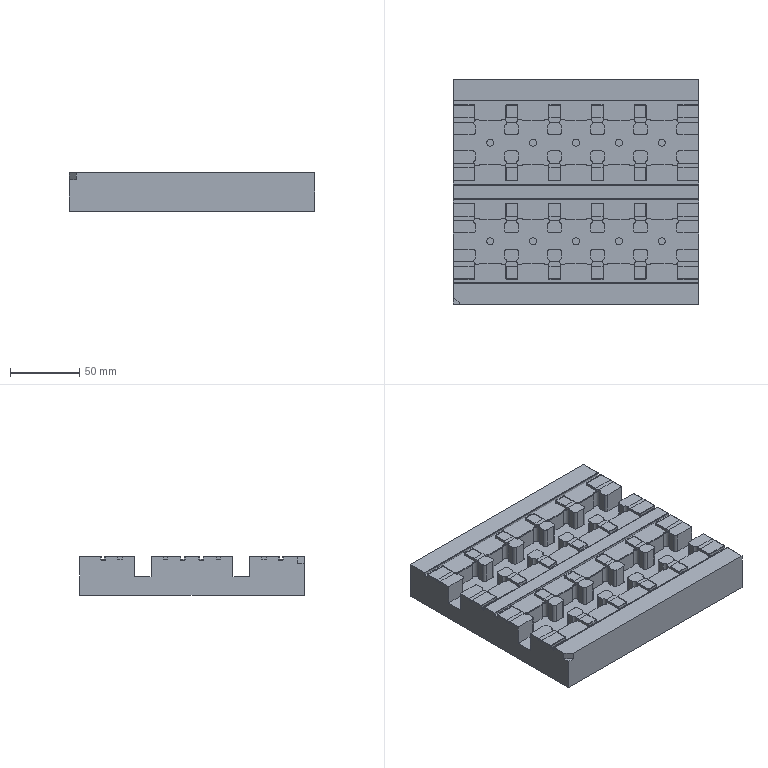NC program | NX | posted by the shop | part box 177 x 162 x 28 mm
Whole program:
%
O0001
(Machine time: 41.67 MIN)
(===Total Tool:4===)
(T2=D17R0.8FlyCutter D=17.  R=0.8  D-  H02 Z=1.    )
(T10=D10    D=10.  R=0.   D10 H10 Z=1.5   )
(T11=D10-J  D=10.  R=0.   D-  H11 Z=1.5   )
(T1=D6ChamferMill   D=6.   R=0.   D-  H01 Z=28.5  )
G80 G90 G17 G49 G40
G91 G28 Z0
M01
N1 T02 M06
(D17R0.8FlyCutter  D=17. R=0.8 H=02 ce=0.20 di=0.10)
(MAX_Z=80. MIN_Z=1. Time=26.18M)
T10
G00 G90 G54 X109. Y-78.971 M03 S2000
G43 H02 Z80.
M08
Z32.3
G01 Z30.3 F3000.
X97.
X-97.
Y-68.441
X97.
Y-57.912
X-97.
Y-47.382
X97.
Y-36.853
X-97.
Y-26.324
X97.
Y-15.794
X-97.
Y-5.265
X97.
Y5.265
X-97.
Y15.794
X97.
Y26.324
X-97.
Y36.853
X97.
Y47.382
X-97.
Y57.912
X97.
Y68.441
X-97.
Y78.971
X97.
X109.
Z32.3
G00 Z33.5
Y-78.971
Z32.1
G01 Z30.1
X97.
X-97.
Y-68.441
X97.
Y-57.912
X-97.
Y-47.382
X97.
Y-36.853
X-97.
Y-26.324
X97.
Y-15.794
X-97.
Y-5.265
X97.
Y5.265
X-97.
Y15.794
X97.
Y26.324
X-97.
Y36.853
X97.
Y47.382
X-97.
Y57.912
X97.
Y68.441
X-97.
Y78.971
X97.
X109.
Z32.1
G00 Z80.
G00 G90 X-97.2 Y75.602 M03 S2000
Z80.
Z31.
G01 Y81.723 Z30.679 F3000.
X-96.795 Y83.722 Z30.572
X-95.937 Y85.572 Z30.465
X-94.673 Y87.173 Z30.359
X-93.072 Y88.437 Z30.252
X-91.222 Y89.295 Z30.145
X-89.223 Y89.7 Z30.038
X-88.5 Z30.
X88.5 Z29.928
G02 X97.2 Y81. Z29.922 I0.0 J-8.7
G01 Y-81. Z29.856
G02 X88.5 Y-89.7 Z29.851 I-8.7 J0.0
G01 X-88.5 Z29.778
G02 X-97.2 Y-81. Z29.773 I0.0 J8.7
G01 Y81. Z29.707
G02 X-88.5 Y89.7 Z29.701 I8.7 J0.0
G01 X88.5 Z29.629
G02 X97.2 Y81. Z29.623 I0.0 J-8.7
G01 Y-81. Z29.557
G02 X88.5 Y-89.7 Z29.552 I-8.7 J0.0
G01 X-88.5 Z29.479
G02 X-97.2 Y-81. Z29.474 I0.0 J8.7
G01 Y81. Z29.408
G02 X-88.5 Y89.7 Z29.402 I8.7 J0.0
G01 X88.5 Z29.33
G02 X97.2 Y81. Z29.324 I0.0 J-8.7
G01 Y-81. Z29.258
G02 X88.5 Y-89.7 Z29.253 I-8.7 J0.0
G01 X-88.5 Z29.18
G02 X-97.2 Y-81. Z29.175 I0.0 J8.7
G01 Y81. Z29.109
G02 X-88.5 Y89.7 Z29.103 I8.7 J0.0
G01 X88.5 Z29.031
G02 X97.2 Y81. Z29.025 I0.0 J-8.7
G01 Y-81. Z28.959
G02 X88.5 Y-89.7 Z28.954 I-8.7 J0.0
G01 X-88.5 Z28.881
G02 X-97.2 Y-81. Z28.876 I0.0 J8.7
G01 Y81. Z28.81
G02 X-88.5 Y89.7 Z28.804 I8.7 J0.0
G01 X88.5 Z28.732
G02 X97.2 Y81. Z28.726 I0.0 J-8.7
G01 Y-81. Z28.66
G02 X88.5 Y-89.7 Z28.655 I-8.7 J0.0
G01 X-88.5 Z28.582
G02 X-97.2 Y-81. Z28.577 I0.0 J8.7
G01 Y81. Z28.511
G02 X-88.5 Y89.7 Z28.505 I8.7 J0.0
G01 X88.5 Z28.433
G02 X97.2 Y81. Z28.427 I0.0 J-8.7
G01 Y-81. Z28.361
G02 X88.5 Y-89.7 Z28.356 I-8.7 J0.0
G01 X-88.5 Z28.283
G02 X-97.2 Y-81. Z28.278 I0.0 J8.7
G01 Y81. Z28.212
G02 X-88.5 Y89.7 Z28.206 I8.7 J0.0
G01 X88.5 Z28.134
G02 X97.2 Y81. Z28.128 I0.0 J-8.7
G01 Y-81. Z28.062
G02 X88.5 Y-89.7 Z28.057 I-8.7 J0.0
G01 X-88.5 Z27.984
G02 X-97.2 Y-81. Z27.979 I0.0 J8.7
G01 Y81. Z27.913
G02 X-88.5 Y89.7 Z27.907 I8.7 J0.0
G01 X88.5 Z27.835
G02 X97.2 Y81. Z27.829 I0.0 J-8.7
G01 Y-81. Z27.763
G02 X88.5 Y-89.7 Z27.758 I-8.7 J0.0
G01 X-88.5 Z27.686
G02 X-97.2 Y-81. Z27.68 I0.0 J8.7
G01 Y81. Z27.614
G02 X-88.5 Y89.7 Z27.608 I8.7 J0.0
G01 X88.5 Z27.536
G02 X97.2 Y81. Z27.53 I0.0 J-8.7
G01 Y-81. Z27.464
G02 X88.5 Y-89.7 Z27.459 I-8.7 J0.0
G01 X-88.5 Z27.387
G02 X-97.2 Y-81. Z27.381 I0.0 J8.7
G01 Y81. Z27.315
G02 X-88.5 Y89.7 Z27.309 I8.7 J0.0
G01 X88.5 Z27.237
G02 X97.2 Y81. Z27.231 I0.0 J-8.7
G01 Y-81. Z27.165
G02 X88.5 Y-89.7 Z27.16 I-8.7 J0.0
G01 X-88.5 Z27.088
G02 X-97.2 Y-81. Z27.082 I0.0 J8.7
G01 Y81. Z27.016
G02 X-88.5 Y89.7 Z27.01 I8.7 J0.0
G01 X88.5 Z26.938
G02 X97.2 Y81. Z26.933 I0.0 J-8.7
G01 Y-81. Z26.866
G02 X88.5 Y-89.7 Z26.861 I-8.7 J0.0
G01 X-88.5 Z26.789
G02 X-97.2 Y-81. Z26.783 I0.0 J8.7
G01 Y81. Z26.717
G02 X-88.5 Y89.7 Z26.711 I8.7 J0.0
G01 X88.5 Z26.639
G02 X97.2 Y81. Z26.634 I0.0 J-8.7
G01 Y-81. Z26.567
G02 X88.5 Y-89.7 Z26.562 I-8.7 J0.0
G01 X-88.5 Z26.49
G02 X-97.2 Y-81. Z26.484 I0.0 J8.7
G01 Y81. Z26.418
G02 X-88.5 Y89.7 Z26.412 I8.7 J0.0
G01 X88.5 Z26.34
G02 X97.2 Y81. Z26.335 I0.0 J-8.7
G01 Y-81. Z26.268
G02 X88.5 Y-89.7 Z26.263 I-8.7 J0.0
G01 X-88.5 Z26.191
G02 X-97.2 Y-81. Z26.185 I0.0 J8.7
G01 Y81. Z26.119
G02 X-88.5 Y89.7 Z26.113 I8.7 J0.0
G01 X88.5 Z26.041
G02 X97.2 Y81. Z26.036 I0.0 J-8.7
G01 Y-81. Z25.969
G02 X88.5 Y-89.7 Z25.964 I-8.7 J0.0
G01 X-88.5 Z25.892
G02 X-97.2 Y-81. Z25.886 I0.0 J8.7
G01 Y81. Z25.82
G02 X-88.5 Y89.7 Z25.814 I8.7 J0.0
G01 X88.5 Z25.742
G02 X97.2 Y81. Z25.737 I0.0 J-8.7
G01 Y-81. Z25.671
G02 X88.5 Y-89.7 Z25.665 I-8.7 J0.0
G01 X-88.5 Z25.593
G02 X-97.2 Y-81. Z25.587 I0.0 J8.7
G01 Y81. Z25.521
G02 X-88.5 Y89.7 Z25.515 I8.7 J0.0
G01 X88.5 Z25.443
G02 X97.2 Y81. Z25.438 I0.0 J-8.7
G01 Y-81. Z25.372
G02 X88.5 Y-89.7 Z25.366 I-8.7 J0.0
G01 X-88.5 Z25.294
G02 X-97.2 Y-81. Z25.288 I0.0 J8.7
G01 Y81. Z25.222
G02 X-88.5 Y89.7 Z25.216 I8.7 J0.0
G01 X88.5 Z25.144
G02 X97.2 Y81. Z25.139 I0.0 J-8.7
G01 Y-81. Z25.073
G02 X88.5 Y-89.7 Z25.067 I-8.7 J0.0
G01 X-88.5 Z24.995
G02 X-97.2 Y-81. Z24.989 I0.0 J8.7
G01 Y81. Z24.923
G02 X-88.5 Y89.7 Z24.918 I8.7 J0.0
G01 X88.5 Z24.845
G02 X97.2 Y81. Z24.84 I0.0 J-8.7
G01 Y-81. Z24.774
G02 X88.5 Y-89.7 Z24.768 I-8.7 J0.0
G01 X-88.5 Z24.696
G02 X-97.2 Y-81. Z24.69 I0.0 J8.7
G01 Y81. Z24.624
G02 X-88.5 Y89.7 Z24.619 I8.7 J0.0
G01 X88.5 Z24.546
G02 X97.2 Y81. Z24.541 I0.0 J-8.7
G01 Y-81. Z24.475
G02 X88.5 Y-89.7 Z24.469 I-8.7 J0.0
G01 X-88.5 Z24.397
G02 X-97.2 Y-81. Z24.391 I0.0 J8.7
G01 Y81. Z24.325
G02 X-88.5 Y89.7 Z24.32 I8.7 J0.0
G01 X88.5 Z24.247
G02 X97.2 Y81. Z24.242 I0.0 J-8.7
G01 Y-81. Z24.176
G02 X88.5 Y-89.7 Z24.17 I-8.7 J0.0
G01 X-88.5 Z24.098
G02 X-97.2 Y-81. Z24.092 I0.0 J8.7
G01 Y81. Z24.026
G02 X-88.5 Y89.7 Z24.021 I8.7 J0.0
G01 X88.5 Z23.948
G02 X97.2 Y81. Z23.943 I0.0 J-8.7
G01 Y-81. Z23.877
G02 X88.5 Y-89.7 Z23.871 I-8.7 J0.0
G01 X-88.5 Z23.799
G02 X-97.2 Y-81. Z23.793 I0.0 J8.7
G01 Y81. Z23.727
G02 X-88.5 Y89.7 Z23.722 I8.7 J0.0
G01 X88.5 Z23.649
G02 X97.2 Y81. Z23.644 I0.0 J-8.7
G01 Y-81. Z23.578
G02 X88.5 Y-89.7 Z23.572 I-8.7 J0.0
G01 X-88.5 Z23.5
G02 X-97.2 Y-81. Z23.494 I0.0 J8.7
G01 Y81. Z23.428
G02 X-88.5 Y89.7 Z23.423 I8.7 J0.0
G01 X88.5 Z23.35
G02 X97.2 Y81. Z23.345 I0.0 J-8.7
G01 Y-81. Z23.279
G02 X88.5 Y-89.7 Z23.273 I-8.7 J0.0
G01 X-88.5 Z23.201
G02 X-97.2 Y-81. Z23.195 I0.0 J8.7
G01 Y81. Z23.129
G02 X-88.5 Y89.7 Z23.124 I8.7 J0.0
G01 X88.5 Z23.051
G02 X97.2 Y81. Z23.046 I0.0 J-8.7
G01 Y-81. Z22.98
G02 X88.5 Y-89.7 Z22.974 I-8.7 J0.0
G01 X-88.5 Z22.902
G02 X-97.2 Y-81. Z22.896 I0.0 J8.7
G01 Y81. Z22.83
G02 X-88.5 Y89.7 Z22.825 I8.7 J0.0
G01 X88.5 Z22.753
G02 X97.2 Y81. Z22.747 I0.0 J-8.7
G01 Y-81. Z22.681
G02 X88.5 Y-89.7 Z22.675 I-8.7 J0.0
G01 X-88.5 Z22.603
G02 X-97.2 Y-81. Z22.597 I0.0 J8.7
G01 Y81. Z22.531
G02 X-88.5 Y89.7 Z22.526 I8.7 J0.0
G01 X88.5 Z22.454
G02 X97.2 Y81. Z22.448 I0.0 J-8.7
G01 Y-81. Z22.382
G02 X88.5 Y-89.7 Z22.376 I-8.7 J0.0
G01 X-88.5 Z22.304
G02 X-97.2 Y-81. Z22.298 I0.0 J8.7
G01 Y81. Z22.232
G02 X-88.5 Y89.7 Z22.227 I8.7 J0.0
G01 X88.5 Z22.155
G02 X97.2 Y81. Z22.149 I0.0 J-8.7
G01 Y-81. Z22.083
G02 X88.5 Y-89.7 Z22.077 I-8.7 J0.0
G01 X-88.5 Z22.005
G02 X-97.2 Y-81. Z22. I0.0 J8.7
G01 Y81. Z21.933
G02 X-88.5 Y89.7 Z21.928 I8.7 J0.0
G01 X88.5 Z21.856
G02 X97.2 Y81. Z21.85 I0.0 J-8.7
G01 Y-81. Z21.784
G02 X88.5 Y-89.7 Z21.778 I-8.7 J0.0
G01 X-88.5 Z21.706
G02 X-97.2 Y-81. Z21.701 I0.0 J8.7
G01 Y81. Z21.634
G02 X-88.5 Y89.7 Z21.629 I8.7 J0.0
G01 X88.5 Z21.557
G02 X97.2 Y81. Z21.551 I0.0 J-8.7
G01 Y-81. Z21.485
G02 X88.5 Y-89.7 Z21.479 I-8.7 J0.0
G01 X-88.5 Z21.407
G02 X-97.2 Y-81. Z21.402 I0.0 J8.7
G01 Y81. Z21.335
G02 X-88.5 Y89.7 Z21.33 I8.7 J0.0
G01 X88.5 Z21.258
G02 X97.2 Y81. Z21.252 I0.0 J-8.7
G01 Y-81. Z21.186
G02 X88.5 Y-89.7 Z21.18 I-8.7 J0.0
G01 X-88.5 Z21.108
G02 X-97.2 Y-81. Z21.103 I0.0 J8.7
G01 Y81. Z21.037
G02 X-88.5 Y89.7 Z21.031 I8.7 J0.0
G01 X88.5 Z20.959
G02 X97.2 Y81. Z20.953 I0.0 J-8.7
G01 Y-81. Z20.887
G02 X88.5 Y-89.7 Z20.881 I-8.7 J0.0
G01 X-88.5 Z20.809
G02 X-97.2 Y-81. Z20.804 I0.0 J8.7
G01 Y81. Z20.738
G02 X-88.5 Y89.7 Z20.732 I8.7 J0.0
G01 X88.5 Z20.66
G02 X97.2 Y81. Z20.654 I0.0 J-8.7
G01 Y-81. Z20.588
G02 X88.5 Y-89.7 Z20.582 I-8.7 J0.0
G01 X-88.5 Z20.51
G02 X-97.2 Y-81. Z20.505 I0.0 J8.7
G01 Y81. Z20.439
G02 X-88.5 Y89.7 Z20.433 I8.7 J0.0
G01 X88.5 Z20.361
G02 X97.2 Y81. Z20.355 I0.0 J-8.7
G01 Y-81. Z20.289
G02 X88.5 Y-89.7 Z20.284 I-8.7 J0.0
G01 X-88.5 Z20.211
G02 X-97.2 Y-81. Z20.206 I0.0 J8.7
G01 Y81. Z20.14
G02 X-88.5 Y89.7 Z20.134 I8.7 J0.0
G01 X88.5 Z20.062
G02 X97.2 Y81. Z20.056 I0.0 J-8.7
G01 Y-81. Z19.99
G02 X88.5 Y-89.7 Z19.985 I-8.7 J0.0
G01 X-88.5 Z19.912
G02 X-97.2 Y-81. Z19.907 I0.0 J8.7
G01 Y81. Z19.841
G02 X-88.5 Y89.7 Z19.835 I8.7 J0.0
G01 X88.5 Z19.763
G02 X97.2 Y81. Z19.757 I0.0 J-8.7
G01 Y-81. Z19.691
G02 X88.5 Y-89.7 Z19.686 I-8.7 J0.0
G01 X-88.5 Z19.613
G02 X-97.2 Y-81. Z19.608 I0.0 J8.7
G01 Y81. Z19.542
G02 X-88.5 Y89.7 Z19.536 I8.7 J0.0
G01 X88.5 Z19.464
G02 X97.2 Y81. Z19.458 I0.0 J-8.7
G01 Y-81. Z19.392
G02 X88.5 Y-89.7 Z19.387 I-8.7 J0.0
G01 X-88.5 Z19.314
G02 X-97.2 Y-81. Z19.309 I0.0 J8.7
G01 Y81. Z19.243
G02 X-88.5 Y89.7 Z19.237 I8.7 J0.0
G01 X88.5 Z19.165
G02 X97.2 Y81. Z19.159 I0.0 J-8.7
G01 Y-81. Z19.093
G02 X88.5 Y-89.7 Z19.088 I-8.7 J0.0
G01 X-88.5 Z19.015
G02 X-97.2 Y-81. Z19.01 I0.0 J8.7
G01 Y81. Z18.944
G02 X-88.5 Y89.7 Z18.938 I8.7 J0.0
G01 X88.5 Z18.866
G02 X97.2 Y81. Z18.86 I0.0 J-8.7
G01 Y-81. Z18.794
G02 X88.5 Y-89.7 Z18.789 I-8.7 J0.0
G01 X-88.5 Z18.716
G02 X-97.2 Y-81. Z18.711 I0.0 J8.7
G01 Y81. Z18.645
G02 X-88.5 Y89.7 Z18.639 I8.7 J0.0
G01 X88.5 Z18.567
G02 X97.2 Y81. Z18.561 I0.0 J-8.7
G01 Y-81. Z18.495
G02 X88.5 Y-89.7 Z18.49 I-8.7 J0.0
G01 X-88.5 Z18.417
G02 X-97.2 Y-81. Z18.412 I0.0 J8.7
G01 Y81. Z18.346
G02 X-88.5 Y89.7 Z18.34 I8.7 J0.0
G01 X88.5 Z18.268
G02 X97.2 Y81. Z18.262 I0.0 J-8.7
G01 Y-81. Z18.196
G02 X88.5 Y-89.7 Z18.191 I-8.7 J0.0
G01 X-88.5 Z18.118
G02 X-97.2 Y-81. Z18.113 I0.0 J8.7
G01 Y81. Z18.047
G02 X-88.5 Y89.7 Z18.041 I8.7 J0.0
G01 X88.5 Z17.969
G02 X97.2 Y81. Z17.963 I0.0 J-8.7
G01 Y-81. Z17.897
G02 X88.5 Y-89.7 Z17.892 I-8.7 J0.0
G01 X-88.5 Z17.82
G02 X-97.2 Y-81. Z17.814 I0.0 J8.7
G01 Y81. Z17.748
G02 X-88.5 Y89.7 Z17.742 I8.7 J0.0
G01 X88.5 Z17.67
G02 X97.2 Y81. Z17.664 I0.0 J-8.7
G01 Y-81. Z17.598
G02 X88.5 Y-89.7 Z17.593 I-8.7 J0.0
G01 X-88.5 Z17.521
G02 X-97.2 Y-81. Z17.515 I0.0 J8.7
G01 Y81. Z17.449
G02 X-88.5 Y89.7 Z17.443 I8.7 J0.0
G01 X88.5 Z17.371
G02 X97.2 Y81. Z17.365 I0.0 J-8.7
G01 Y-81. Z17.299
G02 X88.5 Y-89.7 Z17.294 I-8.7 J0.0
G01 X-88.5 Z17.222
G02 X-97.2 Y-81. Z17.216 I0.0 J8.7
G01 Y81. Z17.15
G02 X-88.5 Y89.7 Z17.144 I8.7 J0.0
G01 X88.5 Z17.072
G02 X97.2 Y81. Z17.067 I0.0 J-8.7
G01 Y-81. Z17.
G02 X88.5 Y-89.7 Z16.995 I-8.7 J0.0
G01 X-88.5 Z16.923
G02 X-97.2 Y-81. Z16.917 I0.0 J8.7
G01 Y81. Z16.851
G02 X-88.5 Y89.7 Z16.845 I8.7 J0.0
G01 X88.5 Z16.773
G02 X97.2 Y81. Z16.768 I0.0 J-8.7
G01 Y-81. Z16.701
G02 X88.5 Y-89.7 Z16.696 I-8.7 J0.0
G01 X-88.5 Z16.624
G02 X-97.2 Y-81. Z16.618 I0.0 J8.7
G01 Y81. Z16.552
G02 X-88.5 Y89.7 Z16.546 I8.7 J0.0
G01 X88.5 Z16.474
G02 X97.2 Y81. Z16.469 I0.0 J-8.7
G01 Y-81. Z16.402
G02 X88.5 Y-89.7 Z16.397 I-8.7 J0.0
G01 X-88.5 Z16.325
G02 X-97.2 Y-81. Z16.319 I0.0 J8.7
G01 Y81. Z16.253
G02 X-88.5 Y89.7 Z16.247 I8.7 J0.0
G01 X88.5 Z16.175
G02 X97.2 Y81. Z16.17 I0.0 J-8.7
G01 Y-81. Z16.104
G02 X88.5 Y-89.7 Z16.098 I-8.7 J0.0
G01 X-88.5 Z16.026
G02 X-97.2 Y-81. Z16.02 I0.0 J8.7
G01 Y81. Z15.954
G02 X-88.5 Y89.7 Z15.948 I8.7 J0.0
G01 X88.5 Z15.876
G02 X97.2 Y81. Z15.871 I0.0 J-8.7
G01 Y-81. Z15.805
G02 X88.5 Y-89.7 Z15.799 I-8.7 J0.0
G01 X-88.5 Z15.727
G02 X-97.2 Y-81. Z15.721 I0.0 J8.7
G01 Y81. Z15.655
G02 X-88.5 Y89.7 Z15.649 I8.7 J0.0
G01 X88.5 Z15.577
G02 X97.2 Y81. Z15.572 I0.0 J-8.7
G01 Y-81. Z15.506
G02 X88.5 Y-89.7 Z15.5 I-8.7 J0.0
G01 X-88.5 Z15.428
G02 X-97.2 Y-81. Z15.422 I0.0 J8.7
G01 Y81. Z15.356
G02 X-88.5 Y89.7 Z15.351 I8.7 J0.0
G01 X88.5 Z15.278
G02 X97.2 Y81. Z15.273 I0.0 J-8.7
G01 Y-81. Z15.207
G02 X88.5 Y-89.7 Z15.201 I-8.7 J0.0
G01 X-88.5 Z15.129
G02 X-97.2 Y-81. Z15.123 I0.0 J8.7
G01 Y81. Z15.057
G02 X-88.5 Y89.7 Z15.052 I8.7 J0.0
G01 X88.5 Z14.979
G02 X97.2 Y81. Z14.974 I0.0 J-8.7
G01 Y-81. Z14.908
G02 X88.5 Y-89.7 Z14.902 I-8.7 J0.0
G01 X-88.5 Z14.83
G02 X-97.2 Y-81. Z14.824 I0.0 J8.7
G01 Y81. Z14.758
G02 X-88.5 Y89.7 Z14.753 I8.7 J0.0
G01 X88.5 Z14.68
G02 X97.2 Y81. Z14.675 I0.0 J-8.7
G01 Y-81. Z14.609
G02 X88.5 Y-89.7 Z14.603 I-8.7 J0.0
G01 X-88.5 Z14.531
G02 X-97.2 Y-81. Z14.525 I0.0 J8.7
G01 Y81. Z14.459
G02 X-88.5 Y89.7 Z14.454 I8.7 J0.0
G01 X88.5 Z14.381
G02 X97.2 Y81. Z14.376 I0.0 J-8.7
G01 Y-81. Z14.31
G02 X88.5 Y-89.7 Z14.304 I-8.7 J0.0
G01 X-88.5 Z14.232
G02 X-97.2 Y-81. Z14.226 I0.0 J8.7
G01 Y81. Z14.16
G02 X-88.5 Y89.7 Z14.155 I8.7 J0.0
G01 X88.5 Z14.082
G02 X97.2 Y81. Z14.077 I0.0 J-8.7
G01 Y-81. Z14.011
G02 X88.5 Y-89.7 Z14.005 I-8.7 J0.0
G01 X-88.5 Z13.933
G02 X-97.2 Y-81. Z13.927 I0.0 J8.7
G01 Y81. Z13.861
G02 X-88.5 Y89.7 Z13.856 I8.7 J0.0
G01 X88.5 Z13.783
G02 X97.2 Y81. Z13.778 I0.0 J-8.7
G01 Y-81. Z13.712
G02 X88.5 Y-89.7 Z13.706 I-8.7 J0.0
G01 X-88.5 Z13.634
G02 X-97.2 Y-81. Z13.628 I0.0 J8.7
G01 Y81. Z13.562
G02 X-88.5 Y89.7 Z13.557 I8.7 J0.0
G01 X88.5 Z13.484
G02 X97.2 Y81. Z13.479 I0.0 J-8.7
G01 Y-81. Z13.413
G02 X88.5 Y-89.7 Z13.407 I-8.7 J0.0
G01 X-88.5 Z13.335
G02 X-97.2 Y-81. Z13.329 I0.0 J8.7
G01 Y81. Z13.263
G02 X-88.5 Y89.7 Z13.258 I8.7 J0.0
G01 X88.5 Z13.186
G02 X97.2 Y81. Z13.18 I0.0 J-8.7
G01 Y-81. Z13.114
G02 X88.5 Y-89.7 Z13.108 I-8.7 J0.0
G01 X-88.5 Z13.036
G02 X-97.2 Y-81. Z13.03 I0.0 J8.7
G01 Y81. Z12.964
G02 X-88.5 Y89.7 Z12.959 I8.7 J0.0
G01 X88.5 Z12.887
G02 X97.2 Y81. Z12.881 I0.0 J-8.7
G01 Y-81. Z12.815
G02 X88.5 Y-89.7 Z12.809 I-8.7 J0.0
G01 X-88.5 Z12.737
G02 X-97.2 Y-81. Z12.731 I0.0 J8.7
G01 Y81. Z12.665
G02 X-88.5 Y89.7 Z12.66 I8.7 J0.0
G01 X88.5 Z12.588
G02 X97.2 Y81. Z12.582 I0.0 J-8.7
G01 Y-81. Z12.516
G02 X88.5 Y-89.7 Z12.51 I-8.7 J0.0
G01 X-88.5 Z12.438
G02 X-97.2 Y-81. Z12.433 I0.0 J8.7
G01 Y81. Z12.366
G02 X-88.5 Y89.7 Z12.361 I8.7 J0.0
G01 X88.5 Z12.289
G02 X97.2 Y81. Z12.283 I0.0 J-8.7
G01 Y-81. Z12.217
G02 X88.5 Y-89.7 Z12.211 I-8.7 J0.0
G01 X-88.5 Z12.139
G02 X-97.2 Y-81. Z12.134 I0.0 J8.7
G01 Y81. Z12.067
G02 X-88.5 Y89.7 Z12.062 I8.7 J0.0
G01 X88.5 Z11.99
G02 X97.2 Y81. Z11.984 I0.0 J-8.7
G01 Y-81. Z11.918
G02 X88.5 Y-89.7 Z11.912 I-8.7 J0.0
G01 X-88.5 Z11.84
G02 X-97.2 Y-81. Z11.835 I0.0 J8.7
G01 Y81. Z11.768
G02 X-88.5 Y89.7 Z11.763 I8.7 J0.0
G01 X88.5 Z11.691
G02 X97.2 Y81. Z11.685 I0.0 J-8.7
G01 Y-81. Z11.619
G02 X88.5 Y-89.7 Z11.613 I-8.7 J0.0
G01 X-88.5 Z11.541
G02 X-97.2 Y-81. Z11.536 I0.0 J8.7
G01 Y81. Z11.469
G02 X-88.5 Y89.7 Z11.464 I8.7 J0.0
G01 X88.5 Z11.392
G02 X97.2 Y81. Z11.386 I0.0 J-8.7
G01 Y-81. Z11.32
G02 X88.5 Y-89.7 Z11.314 I-8.7 J0.0
G01 X-88.5 Z11.242
G02 X-97.2 Y-81. Z11.237 I0.0 J8.7
G01 Y81. Z11.171
G02 X-88.5 Y89.7 Z11.165 I8.7 J0.0
G01 X88.5 Z11.093
G02 X97.2 Y81. Z11.087 I0.0 J-8.7
G01 Y-81. Z11.021
G02 X88.5 Y-89.7 Z11.015 I-8.7 J0.0
G01 X-88.5 Z10.943
G02 X-97.2 Y-81. Z10.938 I0.0 J8.7
G01 Y81. Z10.872
G02 X-88.5 Y89.7 Z10.866 I8.7 J0.0
G01 X88.5 Z10.794
G02 X97.2 Y81. Z10.788 I0.0 J-8.7
G01 Y-81. Z10.722
G02 X88.5 Y-89.7 Z10.716 I-8.7 J0.0
G01 X-88.5 Z10.644
G02 X-97.2 Y-81. Z10.639 I0.0 J8.7
G01 Y81. Z10.573
G02 X-88.5 Y89.7 Z10.567 I8.7 J0.0
G01 X88.5 Z10.495
G02 X97.2 Y81. Z10.489 I0.0 J-8.7
G01 Y-81. Z10.423
G02 X88.5 Y-89.7 Z10.418 I-8.7 J0.0
G01 X-88.5 Z10.345
G02 X-97.2 Y-81. Z10.34 I0.0 J8.7
G01 Y81. Z10.274
G02 X-88.5 Y89.7 Z10.268 I8.7 J0.0
G01 X88.5 Z10.196
G02 X97.2 Y81. Z10.19 I0.0 J-8.7
G01 Y-81. Z10.124
G02 X88.5 Y-89.7 Z10.119 I-8.7 J0.0
G01 X-88.5 Z10.046
G02 X-97.2 Y-81. Z10.041 I0.0 J8.7
G01 Y81. Z9.975
G02 X-88.5 Y89.7 Z9.969 I8.7 J0.0
G01 X88.5 Z9.897
G02 X97.2 Y81. Z9.891 I0.0 J-8.7
G01 Y-81. Z9.825
G02 X88.5 Y-89.7 Z9.82 I-8.7 J0.0
G01 X-88.5 Z9.747
G02 X-97.2 Y-81. Z9.742 I0.0 J8.7
G01 Y81. Z9.676
G02 X-88.5 Y89.7 Z9.67 I8.7 J0.0
G01 X88.5 Z9.598
G02 X97.2 Y81. Z9.592 I0.0 J-8.7
G01 Y-81. Z9.526
G02 X88.5 Y-89.7 Z9.521 I-8.7 J0.0
G01 X-88.5 Z9.448
G02 X-97.2 Y-81. Z9.443 I0.0 J8.7
G01 Y81. Z9.377
G02 X-88.5 Y89.7 Z9.371 I8.7 J0.0
G01 X88.5 Z9.299
G02 X97.2 Y81. Z9.293 I0.0 J-8.7
G01 Y-81. Z9.227
G02 X88.5 Y-89.7 Z9.222 I-8.7 J0.0
G01 X-88.5 Z9.149
G02 X-97.2 Y-81. Z9.144 I0.0 J8.7
G01 Y81. Z9.078
G02 X-88.5 Y89.7 Z9.072 I8.7 J0.0
G01 X88.5 Z9.
G02 X97.2 Y81. Z8.994 I0.0 J-8.7
G01 Y-81. Z8.928
G02 X88.5 Y-89.7 Z8.923 I-8.7 J0.0
G01 X-88.5 Z8.85
G02 X-97.2 Y-81. Z8.845 I0.0 J8.7
G01 Y81. Z8.779
G02 X-88.5 Y89.7 Z8.773 I8.7 J0.0
G01 X88.5 Z8.701
G02 X97.2 Y81. Z8.695 I0.0 J-8.7
G01 Y-81. Z8.629
G02 X88.5 Y-89.7 Z8.624 I-8.7 J0.0
G01 X-88.5 Z8.551
G02 X-97.2 Y-81. Z8.546 I0.0 J8.7
G01 Y81. Z8.48
G02 X-88.5 Y89.7 Z8.474 I8.7 J0.0
G01 X88.5 Z8.402
G02 X97.2 Y81. Z8.396 I0.0 J-8.7
G01 Y-81. Z8.33
G02 X88.5 Y-89.7 Z8.325 I-8.7 J0.0
G01 X-88.5 Z8.253
G02 X-97.2 Y-81. Z8.247 I0.0 J8.7
G01 Y81. Z8.181
G02 X-88.5 Y89.7 Z8.175 I8.7 J0.0
G01 X88.5 Z8.103
G02 X97.2 Y81. Z8.097 I0.0 J-8.7
G01 Y-81. Z8.031
G02 X88.5 Y-89.7 Z8.026 I-8.7 J0.0
G01 X-88.5 Z7.954
G02 X-97.2 Y-81. Z7.948 I0.0 J8.7
G01 Y81. Z7.882
G02 X-88.5 Y89.7 Z7.876 I8.7 J0.0
G01 X88.5 Z7.804
G02 X97.2 Y81. Z7.798 I0.0 J-8.7
G01 Y-81. Z7.732
G02 X88.5 Y-89.7 Z7.727 I-8.7 J0.0
G01 X-88.5 Z7.655
G02 X-97.2 Y-81. Z7.649 I0.0 J8.7
G01 Y81. Z7.583
G02 X-88.5 Y89.7 Z7.577 I8.7 J0.0
G01 X88.5 Z7.505
G02 X97.2 Y81. Z7.5 I0.0 J-8.7
G01 Y-81. Z7.433
G02 X88.5 Y-89.7 Z7.428 I-8.7 J0.0
G01 X-88.5 Z7.356
G02 X-97.2 Y-81. Z7.35 I0.0 J8.7
G01 Y81. Z7.284
G02 X-88.5 Y89.7 Z7.278 I8.7 J0.0
G01 X88.5 Z7.206
G02 X97.2 Y81. Z7.201 I0.0 J-8.7
G01 Y-81. Z7.134
G02 X88.5 Y-89.7 Z7.129 I-8.7 J0.0
G01 X-88.5 Z7.057
G02 X-97.2 Y-81. Z7.051 I0.0 J8.7
G01 Y81. Z6.985
G02 X-88.5 Y89.7 Z6.979 I8.7 J0.0
G01 X88.5 Z6.907
G02 X97.2 Y81. Z6.902 I0.0 J-8.7
G01 Y-81. Z6.835
G02 X88.5 Y-89.7 Z6.83 I-8.7 J0.0
G01 X-88.5 Z6.758
G02 X-97.2 Y-81. Z6.752 I0.0 J8.7
G01 Y81. Z6.686
G02 X-88.5 Y89.7 Z6.68 I8.7 J0.0
G01 X88.5 Z6.608
G02 X97.2 Y81. Z6.603 I0.0 J-8.7
G01 Y-81. Z6.537
G02 X88.5 Y-89.7 Z6.531 I-8.7 J0.0
G01 X-88.5 Z6.459
G02 X-97.2 Y-81. Z6.453 I0.0 J8.7
G01 Y81. Z6.387
G02 X-88.5 Y89.7 Z6.381 I8.7 J0.0
G01 X88.5 Z6.309
G02 X97.2 Y81. Z6.304 I0.0 J-8.7
G01 Y-81. Z6.238
G02 X88.5 Y-89.7 Z6.232 I-8.7 J0.0
G01 X-88.5 Z6.16
G02 X-97.2 Y-81. Z6.154 I0.0 J8.7
G01 Y81. Z6.088
G02 X-88.5 Y89.7 Z6.082 I8.7 J0.0
G01 X88.5 Z6.01
G02 X97.2 Y81. Z6.005 I0.0 J-8.7
G01 Y-81. Z5.939
G02 X88.5 Y-89.7 Z5.933 I-8.7 J0.0
G01 X-88.5 Z5.861
G02 X-97.2 Y-81. Z5.855 I0.0 J8.7
G01 Y81. Z5.789
G02 X-88.5 Y89.7 Z5.784 I8.7 J0.0
G01 X88.5 Z5.711
G02 X97.2 Y81. Z5.706 I0.0 J-8.7
G01 Y-81. Z5.64
G02 X88.5 Y-89.7 Z5.634 I-8.7 J0.0
G01 X-88.5 Z5.562
G02 X-97.2 Y-81. Z5.556 I0.0 J8.7
G01 Y81. Z5.49
G02 X-88.5 Y89.7 Z5.485 I8.7 J0.0
G01 X88.5 Z5.412
G02 X97.2 Y81. Z5.407 I0.0 J-8.7
G01 Y-81. Z5.341
G02 X88.5 Y-89.7 Z5.335 I-8.7 J0.0
G01 X-88.5 Z5.263
G02 X-97.2 Y-81. Z5.257 I0.0 J8.7
G01 Y81. Z5.191
G02 X-88.5 Y89.7 Z5.186 I8.7 J0.0
G01 X88.5 Z5.113
G02 X97.2 Y81. Z5.108 I0.0 J-8.7
G01 Y-81. Z5.042
G02 X88.5 Y-89.7 Z5.036 I-8.7 J0.0
G01 X-88.5 Z4.964
G02 X-97.2 Y-81. Z4.958 I0.0 J8.7
G01 Y81. Z4.892
G02 X-88.5 Y89.7 Z4.887 I8.7 J0.0
G01 X88.5 Z4.814
G02 X97.2 Y81. Z4.809 I0.0 J-8.7
G01 Y-81. Z4.743
G02 X88.5 Y-89.7 Z4.737 I-8.7 J0.0
G01 X-88.5 Z4.665
G02 X-97.2 Y-81. Z4.659 I0.0 J8.7
G01 Y81. Z4.593
G02 X-88.5 Y89.7 Z4.588 I8.7 J0.0
G01 X88.5 Z4.515
G02 X97.2 Y81. Z4.51 I0.0 J-8.7
G01 Y-81. Z4.444
G02 X88.5 Y-89.7 Z4.438 I-8.7 J0.0
G01 X-88.5 Z4.366
G02 X-97.2 Y-81. Z4.36 I0.0 J8.7
G01 Y81. Z4.294
G02 X-88.5 Y89.7 Z4.289 I8.7 J0.0
G01 X88.5 Z4.216
G02 X97.2 Y81. Z4.211 I0.0 J-8.7
G01 Y-81. Z4.145
G02 X88.5 Y-89.7 Z4.139 I-8.7 J0.0
G01 X-88.5 Z4.067
G02 X-97.2 Y-81. Z4.061 I0.0 J8.7
G01 Y81. Z3.995
G02 X-88.5 Y89.7 Z3.99 I8.7 J0.0
G01 X88.5 Z3.917
G02 X97.2 Y81. Z3.912 I0.0 J-8.7
G01 Y-81. Z3.846
G02 X88.5 Y-89.7 Z3.84 I-8.7 J0.0
G01 X-88.5 Z3.768
G02 X-97.2 Y-81. Z3.762 I0.0 J8.7
G01 Y81. Z3.696
G02 X-88.5 Y89.7 Z3.691 I8.7 J0.0
G01 X88.5 Z3.618
G02 X97.2 Y81. Z3.613 I0.0 J-8.7
G01 Y-81. Z3.547
G02 X88.5 Y-89.7 Z3.541 I-8.7 J0.0
G01 X-88.5 Z3.469
G02 X-97.2 Y-81. Z3.463 I0.0 J8.7
G01 Y81. Z3.397
G02 X-88.5 Y89.7 Z3.392 I8.7 J0.0
G01 X88.5 Z3.32
G02 X97.2 Y81. Z3.314 I0.0 J-8.7
G01 Y-81. Z3.248
G02 X88.5 Y-89.7 Z3.242 I-8.7 J0.0
G01 X-88.5 Z3.17
G02 X-97.2 Y-81. Z3.164 I0.0 J8.7
G01 Y81. Z3.098
G02 X-88.5 Y89.7 Z3.093 I8.7 J0.0
G01 X88.5 Z3.021
G02 X97.2 Y81. Z3.015 I0.0 J-8.7
G01 Y-81. Z2.949
G02 X88.5 Y-89.7 Z2.943 I-8.7 J0.0
G01 X-88.5 Z2.871
G02 X-97.2 Y-81. Z2.865 I0.0 J8.7
G01 Y81. Z2.799
G02 X-88.5 Y89.7 Z2.794 I8.7 J0.0
G01 X88.5 Z2.722
G02 X97.2 Y81. Z2.716 I0.0 J-8.7
G01 Y-81. Z2.65
G02 X88.5 Y-89.7 Z2.644 I-8.7 J0.0
G01 X-88.5 Z2.572
G02 X-97.2 Y-81. Z2.567 I0.0 J8.7
G01 Y81. Z2.5
G02 X-88.5 Y89.7 Z2.495 I8.7 J0.0
G01 X88.5 Z2.423
G02 X97.2 Y81. Z2.417 I0.0 J-8.7
G01 Y-81. Z2.351
G02 X88.5 Y-89.7 Z2.345 I-8.7 J0.0
G01 X-88.5 Z2.273
G02 X-97.2 Y-81. Z2.268 I0.0 J8.7
G01 Y81. Z2.201
G02 X-88.5 Y89.7 Z2.196 I8.7 J0.0
G01 X88.5 Z2.124
G02 X97.2 Y81. Z2.118 I0.0 J-8.7
G01 Y-81. Z2.052
G02 X88.5 Y-89.7 Z2.046 I-8.7 J0.0
G01 X-88.5 Z1.974
G02 X-97.2 Y-81. Z1.969 I0.0 J8.7
G01 Y81. Z1.902
G02 X-88.5 Y89.7 Z1.897 I8.7 J0.0
G01 X88.5 Z1.825
G02 X97.2 Y81. Z1.819 I0.0 J-8.7
G01 Y-81. Z1.753
G02 X88.5 Y-89.7 Z1.747 I-8.7 J0.0
G01 X-88.5 Z1.675
G02 X-97.2 Y-81. Z1.67 I0.0 J8.7
G01 Y81. Z1.604
G02 X-88.5 Y89.7 Z1.598 I8.7 J0.0
G01 X88.5 Z1.526
G02 X97.2 Y81. Z1.52 I0.0 J-8.7
G01 Y-81. Z1.454
G02 X88.5 Y-89.7 Z1.448 I-8.7 J0.0
G01 X-88.5 Z1.376
G02 X-97.2 Y-81. Z1.371 I0.0 J8.7
G01 Y81. Z1.305
G02 X-88.5 Y89.7 Z1.299 I8.7 J0.0
G01 X88.5 Z1.227
G02 X97.2 Y81. Z1.221 I0.0 J-8.7
G01 Y-81. Z1.155
G02 X88.5 Y-89.7 Z1.149 I-8.7 J0.0
G01 X-88.5 Z1.077
G02 X-97.2 Y-81. Z1.072 I0.0 J8.7
G01 Y81. Z1.006
G02 X-88.5 Y89.7 Z1. I8.7 J0.0
G01 X88.5
G02 X97.2 Y81. I0.0 J-8.7
G01 Y-81.
G02 X88.5 Y-89.7 I-8.7 J0.0
G01 X-88.5
G02 X-97.2 Y-81. I0.0 J8.7
G01 Y81.
G02 X-88.5 Y89.7 I8.7 J0.0
G01 X-88.1
Z2.
G00 Z80.
G91 G28 Z0.0
M05
M09
G91 G28 Z0.0
M01
N2 T10 M06
(D10  D=10. R=0. H=10 ce=0.05 di=0.30)
(D.N=10 MAX_Z=80. MIN_Z=1.5 Time=2.87M)
T11
G00 G90 G54 X-89.532 Y86.944 M03 S3000
G43 H10 Z80.
M08
Z25.75
G01 Z25.25 F1500.
G41 D10
X-89.327 Y86.488
G03 X-88.5 Y86.05 I.827 J.562
G01 X88.5
G02 X93.55 Y81. I0.0 J-5.05
G01 Y-81.
G02 X88.5 Y-86.05 I-5.05 J0.0
G01 X-88.5
G02 X-93.55 Y-81. I0.0 J5.05
G01 Y81.
G02 X-88.5 Y86.05 I5.05 J0.0
G01 X-88.
G03 X-87.134 Y86.55 I0.0 J1.
G01 G40 X-86.963 Y87.02
Z25.75
G00 Z30.5
X-89.532 Y86.944
Z21.
G01 Z20.5
G41 D10
X-89.327 Y86.488
G03 X-88.5 Y86.05 I.827 J.562
G01 X88.5
G02 X93.55 Y81. I0.0 J-5.05
G01 Y-81.
G02 X88.5 Y-86.05 I-5.05 J0.0
G01 X-88.5
G02 X-93.55 Y-81. I0.0 J5.05
G01 Y81.
G02 X-88.5 Y86.05 I5.05 J0.0
G01 X-88.
G03 X-87.134 Y86.55 I0.0 J1.
G01 G40 X-86.963 Y87.02
Z21.
G00 Z25.75
X-89.532 Y86.944
Z16.25
G01 Z15.75
G41 D10
X-89.327 Y86.488
G03 X-88.5 Y86.05 I.827 J.562
G01 X88.5
G02 X93.55 Y81. I0.0 J-5.05
G01 Y-81.
G02 X88.5 Y-86.05 I-5.05 J0.0
G01 X-88.5
G02 X-93.55 Y-81. I0.0 J5.05
G01 Y81.
G02 X-88.5 Y86.05 I5.05 J0.0
G01 X-88.
G03 X-87.134 Y86.55 I0.0 J1.
G01 G40 X-86.963 Y87.02
Z16.25
G00 Z21.
X-89.532 Y86.944
Z11.5
G01 Z11.
G41 D10
X-89.327 Y86.488
G03 X-88.5 Y86.05 I.827 J.562
G01 X88.5
G02 X93.55 Y81. I0.0 J-5.05
G01 Y-81.
G02 X88.5 Y-86.05 I-5.05 J0.0
G01 X-88.5
G02 X-93.55 Y-81. I0.0 J5.05
G01 Y81.
G02 X-88.5 Y86.05 I5.05 J0.0
G01 X-88.
G03 X-87.134 Y86.55 I0.0 J1.
G01 G40 X-86.963 Y87.02
Z11.5
G00 Z16.25
X-89.532 Y86.944
Z6.75
G01 Z6.25
G41 D10
X-89.327 Y86.488
G03 X-88.5 Y86.05 I.827 J.562
G01 X88.5
G02 X93.55 Y81. I0.0 J-5.05
G01 Y-81.
G02 X88.5 Y-86.05 I-5.05 J0.0
G01 X-88.5
G02 X-93.55 Y-81. I0.0 J5.05
G01 Y81.
G02 X-88.5 Y86.05 I5.05 J0.0
G01 X-88.
G03 X-87.134 Y86.55 I0.0 J1.
G01 G40 X-86.963 Y87.02
Z6.75
G00 Z11.5
X-89.532 Y86.944
Z2.
G01 Z1.5
G41 D10
X-89.327 Y86.488
G03 X-88.5 Y86.05 I.827 J.562
G01 X88.5
G02 X93.55 Y81. I0.0 J-5.05
G01 Y-81.
G02 X88.5 Y-86.05 I-5.05 J0.0
G01 X-88.5
G02 X-93.55 Y-81. I0.0 J5.05
G01 Y81.
G02 X-88.5 Y86.05 I5.05 J0.0
G01 X-88.
G03 X-87.134 Y86.55 I0.0 J1.
G01 G40 X-86.963 Y87.02
Z2.
G00 Z80.
G91 G28 Z0.0
M05
M09
G91 G28 Z0.0
M01
N3 T11 M06
(D10-J  D=10. R=0. H=11 ce=0.00 di=0.00)
(MAX_Z=80. MIN_Z=30. Time=6.57M)
T01
G00 G90 G54 X105.5 Y-81.086 M03 S3000
G43 H11 Z80.
M08
Z32.
G01 Z30. F1000.
X93.5
X-93.5
Y-76.171
X93.5
Y-71.257
X-93.5
Y-66.343
X93.5
Y-61.429
X-93.5
Y-56.514
X93.5
Y-51.6
X-93.5
Y-46.686
X93.5
Y-41.771
X-93.5
Y-36.857
X93.5
Y-31.943
X-93.5
Y-27.029
X93.5
Y-22.114
X-93.5
Y-17.2
X93.5
Y-12.286
X-93.5
Y-7.371
X93.5
Y-2.457
X-93.5
Y2.457
X93.5
Y7.371
X-93.5
Y12.286
X93.5
Y17.2
X-93.5
Y22.114
X93.5
Y27.029
X-93.5
Y31.943
X93.5
Y36.857
X-93.5
Y41.771
X93.5
Y46.686
X-93.5
Y51.6
X93.5
Y56.514
X-93.5
Y61.429
X93.5
Y66.343
X-93.5
Y71.257
X93.5
Y76.171
X-93.5
Y81.086
X93.5
X105.5
Z32.
G00 Z80.
G91 G28 Z0.0
M05
M09
G91 G28 Z0.0
M01
N4 T01 M06
(D6ChamferMill  D=6. R=0. H=01 ce=0.00 di=0.00)
(MAX_Z=80. MIN_Z=28.5 Time=0.71M)
T11
G00 G90 G54 X-.25 Y83.128 M03 S3000
G43 H01 Z80.
M08
Z32.099
G01 Z28.5 F1000.
G03 X-.33 Y82.828 I.52 J-.3
X-.03 Y82.308 I.6 J0.0
G01 X0.0 Y82.3
X88.5
G02 X89.8 Y81. I0.0 J-1.3
G01 Y-81.
G02 X88.5 Y-82.3 I-1.3 J0.0
G01 X-88.5
G02 X-89.8 Y-81. I0.0 J1.3
G01 Y81.
G02 X-88.5 Y82.3 I1.3 J0.0
G01 X0.0
X.03 Y82.308
G03 X.33 Y82.828 I-.3 J.52
X.25 Y83.128 I-.6 J0.0
G01 Z32.099
G00 Z80.
G91 G28 Z0.0
M05
M09
G91 G28 Z0.0
M01
N5 T11 M06
(D10-J  D=10. R=0. H=11 ce=0.00 di=0.20)
(D.N=11 MAX_Z=80. MIN_Z=1.5 Time=4.33M)
T02
G00 G90 G54 X89.513 Y-87.126 M03 S3000
G43 H11 Z80.
M08
Z21.
G01 Z20.5 F1000.
G41 D11
X89.497 Y-86.927
G03 X88.5 Y-86.01 I-.997 J-.083
G01 X-88.5
G02 X-93.51 Y-81. I0.0 J5.01
G01 Y81.
G02 X-88.5 Y86.01 I5.01 J0.0
G01 X88.5
G02 X93.51 Y81. I0.0 J-5.01
G01 Y-81.
G02 X88.5 Y-86.01 I-5.01 J0.0
G01 X88.
G03 X87. Y-87.01 I0.0 J-1.
G01 G40 Y-87.21
X89.512 Y-87.126
G41 D11
X89.497 Y-86.927
G03 X88.5 Y-86. I-.997 J-.073
G01 X-88.5
G02 X-93.5 Y-81. I0.0 J5.
G01 Y81.
G02 X-88.5 Y86. I5. J0.0
G01 X88.5
G02 X93.5 Y81. I0.0 J-5.
G01 Y-81.
G02 X88.5 Y-86. I-5. J0.0
G01 X88.
G03 X87. Y-87. I0.0 J-1.
G01 Y-87.01
G40 Y-87.21
Z21.
G00 Z80.
X89.513 Y-87.126
Z11.5
G01 Z11.
G41 D11
X89.497 Y-86.927
G03 X88.5 Y-86.01 I-.997 J-.083
G01 X-88.5
G02 X-93.51 Y-81. I0.0 J5.01
G01 Y81.
G02 X-88.5 Y86.01 I5.01 J0.0
G01 X88.5
G02 X93.51 Y81. I0.0 J-5.01
G01 Y-81.
G02 X88.5 Y-86.01 I-5.01 J0.0
G01 X88.
G03 X87. Y-87.01 I0.0 J-1.
G01 G40 Y-87.21
X89.512 Y-87.126
G41 D11
X89.497 Y-86.927
G03 X88.5 Y-86. I-.997 J-.073
G01 X-88.5
G02 X-93.5 Y-81. I0.0 J5.
G01 Y81.
G02 X-88.5 Y86. I5. J0.0
G01 X88.5
G02 X93.5 Y81. I0.0 J-5.
G01 Y-81.
G02 X88.5 Y-86. I-5. J0.0
G01 X88.
G03 X87. Y-87. I0.0 J-1.
G01 Y-87.01
G40 Y-87.21
Z11.5
G00 Z80.
X89.513 Y-87.126
Z2.
G01 Z1.5
G41 D11
X89.497 Y-86.927
G03 X88.5 Y-86.01 I-.997 J-.083
G01 X-88.5
G02 X-93.51 Y-81. I0.0 J5.01
G01 Y81.
G02 X-88.5 Y86.01 I5.01 J0.0
G01 X88.5
G02 X93.51 Y81. I0.0 J-5.01
G01 Y-81.
G02 X88.5 Y-86.01 I-5.01 J0.0
G01 X88.
G03 X87. Y-87.01 I0.0 J-1.
G01 G40 Y-87.21
X89.512 Y-87.126
G41 D11
X89.497 Y-86.927
G03 X88.5 Y-86. I-.997 J-.073
G01 X-88.5
G02 X-93.5 Y-81. I0.0 J5.
G01 Y81.
G02 X-88.5 Y86. I5. J0.0
G01 X88.5
G02 X93.5 Y81. I0.0 J-5.
G01 Y-81.
G02 X88.5 Y-86. I-5. J0.0
G01 X88.
G03 X87. Y-87. I0.0 J-1.
G01 Y-87.01
G40 Y-87.21
Z2.
G00 Z80.
M05
M09
G91 G28 Z0.0
G91 G28 Y0.0
M30
%